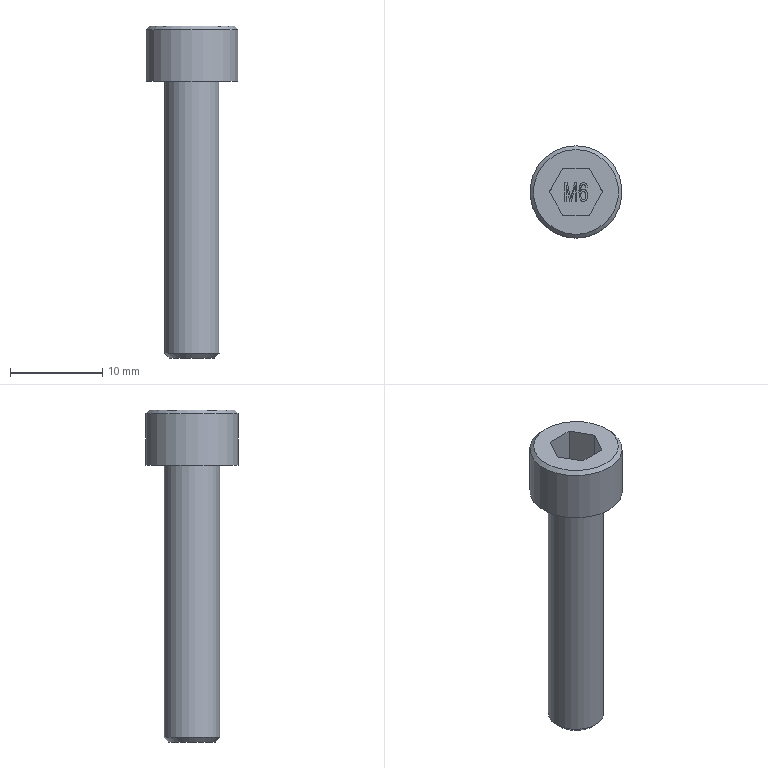Part | STEP file | EM10603000 | 1 solid | 38 faces | box 10 x 10 x 36 mm | volume 1228 mm3 | plane 25 | other 9 | cylinder 2 | cone 2 | commonest cylinder face diameters 6 x1 10 x1